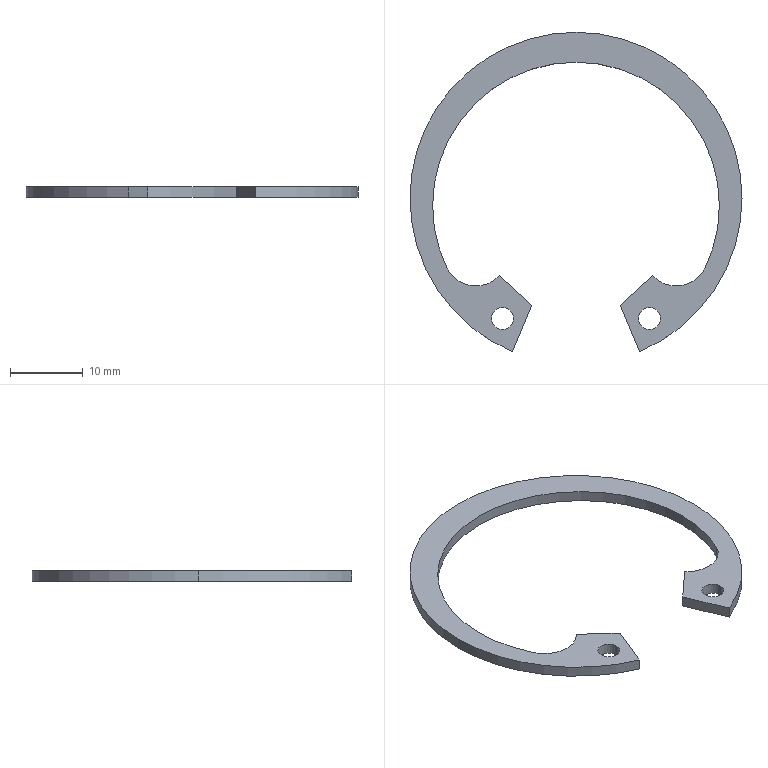Part | STEP file | 1 solid | 18 faces | box 45.5 x 43.768 x 1.5 mm | volume 674.493 mm3 | cylinder 12 | plane 6 | commonest cylinder face diameters 3 x4 39.3 x3 45.5 x3 8.8 x2
STEP:
#1=CARTESIAN_POINT('',(0.,0.,0.));
#2=DIRECTION('',(0.,0.,1.));
#3=DIRECTION('',(1.,0.,0.));
#4=AXIS2_PLACEMENT_3D('',#1,#2,#3);
#5=CARTESIAN_POINT('',(8.568,-16.466,-0.75));
#6=VERTEX_POINT('',#5);
#7=CARTESIAN_POINT('',(11.568,-16.466,-0.75));
#8=VERTEX_POINT('',#7);
#9=CARTESIAN_POINT('',(10.068,-16.466,-0.75));
#10=DIRECTION('',(0.,0.,1.));
#11=DIRECTION('',(-1.,0.,0.));
#12=AXIS2_PLACEMENT_3D('',#9,#10,#11);
#13=CIRCLE('',#12,1.5);
#14=CARTESIAN_POINT('',(0.,0.,-0.75));
#15=DIRECTION('',(0.,0.,1.));
#16=DIRECTION('',(1.,0.,0.));
#17=AXIS2_PLACEMENT_3D('',#14,#15,#16);
#18=PLANE('',#17);
#19=CARTESIAN_POINT('',(10.068,-16.466));
#20=DIRECTION('',(-1.,0.));
#21=AXIS2_PLACEMENT_2D('',#19,#20);
#22=CIRCLE('',#21,1.5);
#23=(GEOMETRIC_REPRESENTATION_CONTEXT(2)PARAMETRIC_REPRESENTATION_CONTEXT()REPRESENTATION_CONTEXT('',''));
#24=DEFINITIONAL_REPRESENTATION('',(#22),#23);
#25=PCURVE('',#18,#24);
#26=CARTESIAN_POINT('',(10.068,-16.466,0.75));
#27=DIRECTION('',(0.,0.,-1.));
#28=DIRECTION('',(-1.,0.,0.));
#29=AXIS2_PLACEMENT_3D('',#26,#27,#28);
#30=CYLINDRICAL_SURFACE('',#29,1.5);
#31=CARTESIAN_POINT('',(6.283,1.5));
#32=DIRECTION('',(-1.,0.));
#33=VECTOR('',#32,1.);
#34=LINE('',#31,#33);
#35=(GEOMETRIC_REPRESENTATION_CONTEXT(2)PARAMETRIC_REPRESENTATION_CONTEXT()REPRESENTATION_CONTEXT('',''));
#36=DEFINITIONAL_REPRESENTATION('',(#34),#35);
#37=PCURVE('',#30,#36);
#38=SURFACE_CURVE('',#13,(#25,#37),.PCURVE_S1.);
#39=EDGE_CURVE('',#6,#8,#38,.T.);
#40=ORIENTED_EDGE('',*,*,#39,.T.);
#41=CARTESIAN_POINT('',(10.068,-16.466,-0.75));
#42=DIRECTION('',(0.,0.,1.));
#43=DIRECTION('',(-1.,0.,0.));
#44=AXIS2_PLACEMENT_3D('',#41,#42,#43);
#45=CIRCLE('',#44,1.5);
#46=CARTESIAN_POINT('',(10.068,-16.466));
#47=DIRECTION('',(-1.,0.));
#48=AXIS2_PLACEMENT_2D('',#46,#47);
#49=CIRCLE('',#48,1.5);
#50=(GEOMETRIC_REPRESENTATION_CONTEXT(2)PARAMETRIC_REPRESENTATION_CONTEXT()REPRESENTATION_CONTEXT('',''));
#51=DEFINITIONAL_REPRESENTATION('',(#49),#50);
#52=PCURVE('',#18,#51);
#53=CARTESIAN_POINT('',(10.068,-16.466,0.75));
#54=DIRECTION('',(0.,0.,-1.));
#55=DIRECTION('',(-1.,0.,0.));
#56=AXIS2_PLACEMENT_3D('',#53,#54,#55);
#57=CYLINDRICAL_SURFACE('',#56,1.5);
#58=CARTESIAN_POINT('',(6.283,1.5));
#59=DIRECTION('',(-1.,0.));
#60=VECTOR('',#59,1.);
#61=LINE('',#58,#60);
#62=(GEOMETRIC_REPRESENTATION_CONTEXT(2)PARAMETRIC_REPRESENTATION_CONTEXT()REPRESENTATION_CONTEXT('',''));
#63=DEFINITIONAL_REPRESENTATION('',(#61),#62);
#64=PCURVE('',#57,#63);
#65=SURFACE_CURVE('',#45,(#52,#64),.PCURVE_S1.);
#66=EDGE_CURVE('',#8,#6,#65,.T.);
#67=ORIENTED_EDGE('',*,*,#66,.T.);
#68=EDGE_LOOP('',(#40,#67));
#69=FACE_BOUND('',#68,.T.);
#70=CARTESIAN_POINT('',(-11.568,-16.466,-0.75));
#71=VERTEX_POINT('',#70);
#72=CARTESIAN_POINT('',(-8.568,-16.466,-0.75));
#73=VERTEX_POINT('',#72);
#74=CARTESIAN_POINT('',(-10.068,-16.466,-0.75));
#75=DIRECTION('',(0.,0.,1.));
#76=DIRECTION('',(-1.,0.,0.));
#77=AXIS2_PLACEMENT_3D('',#74,#75,#76);
#78=CIRCLE('',#77,1.5);
#79=CARTESIAN_POINT('',(-10.068,-16.466));
#80=DIRECTION('',(-1.,0.));
#81=AXIS2_PLACEMENT_2D('',#79,#80);
#82=CIRCLE('',#81,1.5);
#83=(GEOMETRIC_REPRESENTATION_CONTEXT(2)PARAMETRIC_REPRESENTATION_CONTEXT()REPRESENTATION_CONTEXT('',''));
#84=DEFINITIONAL_REPRESENTATION('',(#82),#83);
#85=PCURVE('',#18,#84);
#86=CARTESIAN_POINT('',(-10.068,-16.466,0.75));
#87=DIRECTION('',(0.,0.,-1.));
#88=DIRECTION('',(-1.,0.,0.));
#89=AXIS2_PLACEMENT_3D('',#86,#87,#88);
#90=CYLINDRICAL_SURFACE('',#89,1.5);
#91=CARTESIAN_POINT('',(6.283,1.5));
#92=DIRECTION('',(-1.,0.));
#93=VECTOR('',#92,1.);
#94=LINE('',#91,#93);
#95=(GEOMETRIC_REPRESENTATION_CONTEXT(2)PARAMETRIC_REPRESENTATION_CONTEXT()REPRESENTATION_CONTEXT('',''));
#96=DEFINITIONAL_REPRESENTATION('',(#94),#95);
#97=PCURVE('',#90,#96);
#98=SURFACE_CURVE('',#78,(#85,#97),.PCURVE_S1.);
#99=EDGE_CURVE('',#71,#73,#98,.T.);
#100=ORIENTED_EDGE('',*,*,#99,.T.);
#101=CARTESIAN_POINT('',(-10.068,-16.466,-0.75));
#102=DIRECTION('',(0.,0.,1.));
#103=DIRECTION('',(-1.,0.,0.));
#104=AXIS2_PLACEMENT_3D('',#101,#102,#103);
#105=CIRCLE('',#104,1.5);
#106=CARTESIAN_POINT('',(-10.068,-16.466));
#107=DIRECTION('',(-1.,0.));
#108=AXIS2_PLACEMENT_2D('',#106,#107);
#109=CIRCLE('',#108,1.5);
#110=(GEOMETRIC_REPRESENTATION_CONTEXT(2)PARAMETRIC_REPRESENTATION_CONTEXT()REPRESENTATION_CONTEXT('',''));
#111=DEFINITIONAL_REPRESENTATION('',(#109),#110);
#112=PCURVE('',#18,#111);
#113=CARTESIAN_POINT('',(-10.068,-16.466,0.75));
#114=DIRECTION('',(0.,0.,-1.));
#115=DIRECTION('',(-1.,0.,0.));
#116=AXIS2_PLACEMENT_3D('',#113,#114,#115);
#117=CYLINDRICAL_SURFACE('',#116,1.5);
#118=CARTESIAN_POINT('',(6.283,1.5));
#119=DIRECTION('',(-1.,0.));
#120=VECTOR('',#119,1.);
#121=LINE('',#118,#120);
#122=(GEOMETRIC_REPRESENTATION_CONTEXT(2)PARAMETRIC_REPRESENTATION_CONTEXT()REPRESENTATION_CONTEXT('',''));
#123=DEFINITIONAL_REPRESENTATION('',(#121),#122);
#124=PCURVE('',#117,#123);
#125=SURFACE_CURVE('',#105,(#112,#124),.PCURVE_S1.);
#126=EDGE_CURVE('',#73,#71,#125,.T.);
#127=ORIENTED_EDGE('',*,*,#126,.T.);
#128=EDGE_LOOP('',(#100,#127));
#129=FACE_BOUND('',#128,.T.);
#130=CARTESIAN_POINT('',(8.706,-21.018,-0.75));
#131=VERTEX_POINT('',#130);
#132=CARTESIAN_POINT('',(6.066,-14.643,-0.75));
#133=VERTEX_POINT('',#132);
#134=CARTESIAN_POINT('',(6.066,-14.643,-0.75));
#135=DIRECTION('',(-0.3827,0.9239,0.));
#136=VECTOR('',#135,1.);
#137=LINE('',#134,#136);
#138=CARTESIAN_POINT('',(6.066,-14.643));
#139=DIRECTION('',(-0.3827,0.9239));
#140=VECTOR('',#139,1.);
#141=LINE('',#138,#140);
#142=(GEOMETRIC_REPRESENTATION_CONTEXT(2)PARAMETRIC_REPRESENTATION_CONTEXT()REPRESENTATION_CONTEXT('',''));
#143=DEFINITIONAL_REPRESENTATION('',(#141),#142);
#144=PCURVE('',#18,#143);
#145=CARTESIAN_POINT('',(6.066,-14.643,0.75));
#146=DIRECTION('',(0.9239,0.3827,0.));
#147=DIRECTION('',(0.,0.,-1.));
#148=AXIS2_PLACEMENT_3D('',#145,#146,#147);
#149=PLANE('',#148);
#150=CARTESIAN_POINT('',(1.5,0.));
#151=DIRECTION('',(0.,1.));
#152=VECTOR('',#151,1.);
#153=LINE('',#150,#152);
#154=(GEOMETRIC_REPRESENTATION_CONTEXT(2)PARAMETRIC_REPRESENTATION_CONTEXT()REPRESENTATION_CONTEXT('',''));
#155=DEFINITIONAL_REPRESENTATION('',(#153),#154);
#156=PCURVE('',#149,#155);
#157=SURFACE_CURVE('',#137,(#144,#156),.PCURVE_S1.);
#158=EDGE_CURVE('',#131,#133,#157,.T.);
#159=ORIENTED_EDGE('',*,*,#158,.T.);
#160=CARTESIAN_POINT('',(10.492,-10.593,-0.75));
#161=VERTEX_POINT('',#160);
#162=CARTESIAN_POINT('',(10.492,-10.593,-0.75));
#163=DIRECTION('',(0.7377,0.6752,0.));
#164=VECTOR('',#163,1.);
#165=LINE('',#162,#164);
#166=CARTESIAN_POINT('',(10.492,-10.593));
#167=DIRECTION('',(0.7377,0.6752));
#168=VECTOR('',#167,1.);
#169=LINE('',#166,#168);
#170=(GEOMETRIC_REPRESENTATION_CONTEXT(2)PARAMETRIC_REPRESENTATION_CONTEXT()REPRESENTATION_CONTEXT('',''));
#171=DEFINITIONAL_REPRESENTATION('',(#169),#170);
#172=PCURVE('',#18,#171);
#173=CARTESIAN_POINT('',(10.492,-10.593,0.75));
#174=DIRECTION('',(0.6752,-0.7377,0.));
#175=DIRECTION('',(0.,0.,-1.));
#176=AXIS2_PLACEMENT_3D('',#173,#174,#175);
#177=PLANE('',#176);
#178=CARTESIAN_POINT('',(1.5,0.));
#179=DIRECTION('',(0.,1.));
#180=VECTOR('',#179,1.);
#181=LINE('',#178,#180);
#182=(GEOMETRIC_REPRESENTATION_CONTEXT(2)PARAMETRIC_REPRESENTATION_CONTEXT()REPRESENTATION_CONTEXT('',''));
#183=DEFINITIONAL_REPRESENTATION('',(#181),#182);
#184=PCURVE('',#177,#183);
#185=SURFACE_CURVE('',#165,(#172,#184),.PCURVE_S1.);
#186=EDGE_CURVE('',#133,#161,#185,.T.);
#187=ORIENTED_EDGE('',*,*,#186,.T.);
#188=CARTESIAN_POINT('',(17.701,-9.532,-0.75));
#189=VERTEX_POINT('',#188);
#190=CARTESIAN_POINT('',(13.737,-7.622,-0.75));
#191=DIRECTION('',(0.,0.,1.));
#192=DIRECTION('',(-1.,0.,0.));
#193=AXIS2_PLACEMENT_3D('',#190,#191,#192);
#194=CIRCLE('',#193,4.4);
#195=CARTESIAN_POINT('',(13.737,-7.622));
#196=DIRECTION('',(-1.,0.));
#197=AXIS2_PLACEMENT_2D('',#195,#196);
#198=CIRCLE('',#197,4.4);
#199=(GEOMETRIC_REPRESENTATION_CONTEXT(2)PARAMETRIC_REPRESENTATION_CONTEXT()REPRESENTATION_CONTEXT('',''));
#200=DEFINITIONAL_REPRESENTATION('',(#198),#199);
#201=PCURVE('',#18,#200);
#202=CARTESIAN_POINT('',(13.737,-7.622,0.75));
#203=DIRECTION('',(0.,0.,-1.));
#204=DIRECTION('',(-1.,0.,0.));
#205=AXIS2_PLACEMENT_3D('',#202,#203,#204);
#206=CYLINDRICAL_SURFACE('',#205,4.4);
#207=CARTESIAN_POINT('',(6.283,1.5));
#208=DIRECTION('',(-1.,0.));
#209=VECTOR('',#208,1.);
#210=LINE('',#207,#209);
#211=(GEOMETRIC_REPRESENTATION_CONTEXT(2)PARAMETRIC_REPRESENTATION_CONTEXT()REPRESENTATION_CONTEXT('',''));
#212=DEFINITIONAL_REPRESENTATION('',(#210),#211);
#213=PCURVE('',#206,#212);
#214=SURFACE_CURVE('',#194,(#201,#213),.PCURVE_S1.);
#215=EDGE_CURVE('',#161,#189,#214,.T.);
#216=ORIENTED_EDGE('',*,*,#215,.T.);
#217=CARTESIAN_POINT('',(19.65,-1.,-0.75));
#218=VERTEX_POINT('',#217);
#219=CARTESIAN_POINT('',(0.,-1.,-0.75));
#220=DIRECTION('',(0.,0.,1.));
#221=DIRECTION('',(-1.,0.,0.));
#222=AXIS2_PLACEMENT_3D('',#219,#220,#221);
#223=CIRCLE('',#222,19.65);
#224=CARTESIAN_POINT('',(0.,-1.));
#225=DIRECTION('',(-1.,0.));
#226=AXIS2_PLACEMENT_2D('',#224,#225);
#227=CIRCLE('',#226,19.65);
#228=(GEOMETRIC_REPRESENTATION_CONTEXT(2)PARAMETRIC_REPRESENTATION_CONTEXT()REPRESENTATION_CONTEXT('',''));
#229=DEFINITIONAL_REPRESENTATION('',(#227),#228);
#230=PCURVE('',#18,#229);
#231=CARTESIAN_POINT('',(0.,-1.,0.75));
#232=DIRECTION('',(0.,0.,-1.));
#233=DIRECTION('',(-1.,0.,0.));
#234=AXIS2_PLACEMENT_3D('',#231,#232,#233);
#235=CYLINDRICAL_SURFACE('',#234,19.65);
#236=CARTESIAN_POINT('',(6.283,1.5));
#237=DIRECTION('',(-1.,0.));
#238=VECTOR('',#237,1.);
#239=LINE('',#236,#238);
#240=(GEOMETRIC_REPRESENTATION_CONTEXT(2)PARAMETRIC_REPRESENTATION_CONTEXT()REPRESENTATION_CONTEXT('',''));
#241=DEFINITIONAL_REPRESENTATION('',(#239),#240);
#242=PCURVE('',#235,#241);
#243=SURFACE_CURVE('',#223,(#230,#242),.PCURVE_S1.);
#244=EDGE_CURVE('',#189,#218,#243,.T.);
#245=ORIENTED_EDGE('',*,*,#244,.T.);
#246=CARTESIAN_POINT('',(-19.65,-1.,-0.75));
#247=VERTEX_POINT('',#246);
#248=CARTESIAN_POINT('',(0.,-1.,-0.75));
#249=DIRECTION('',(0.,0.,1.));
#250=DIRECTION('',(-1.,0.,0.));
#251=AXIS2_PLACEMENT_3D('',#248,#249,#250);
#252=CIRCLE('',#251,19.65);
#253=CARTESIAN_POINT('',(0.,-1.));
#254=DIRECTION('',(-1.,0.));
#255=AXIS2_PLACEMENT_2D('',#253,#254);
#256=CIRCLE('',#255,19.65);
#257=(GEOMETRIC_REPRESENTATION_CONTEXT(2)PARAMETRIC_REPRESENTATION_CONTEXT()REPRESENTATION_CONTEXT('',''));
#258=DEFINITIONAL_REPRESENTATION('',(#256),#257);
#259=PCURVE('',#18,#258);
#260=CARTESIAN_POINT('',(0.,-1.,0.75));
#261=DIRECTION('',(0.,0.,-1.));
#262=DIRECTION('',(-1.,0.,0.));
#263=AXIS2_PLACEMENT_3D('',#260,#261,#262);
#264=CYLINDRICAL_SURFACE('',#263,19.65);
#265=CARTESIAN_POINT('',(6.283,1.5));
#266=DIRECTION('',(-1.,0.));
#267=VECTOR('',#266,1.);
#268=LINE('',#265,#267);
#269=(GEOMETRIC_REPRESENTATION_CONTEXT(2)PARAMETRIC_REPRESENTATION_CONTEXT()REPRESENTATION_CONTEXT('',''));
#270=DEFINITIONAL_REPRESENTATION('',(#268),#269);
#271=PCURVE('',#264,#270);
#272=SURFACE_CURVE('',#252,(#259,#271),.PCURVE_S1.);
#273=EDGE_CURVE('',#218,#247,#272,.T.);
#274=ORIENTED_EDGE('',*,*,#273,.T.);
#275=CARTESIAN_POINT('',(-17.701,-9.532,-0.75));
#276=VERTEX_POINT('',#275);
#277=CARTESIAN_POINT('',(0.,-1.,-0.75));
#278=DIRECTION('',(0.,0.,1.));
#279=DIRECTION('',(-1.,0.,0.));
#280=AXIS2_PLACEMENT_3D('',#277,#278,#279);
#281=CIRCLE('',#280,19.65);
#282=CARTESIAN_POINT('',(0.,-1.));
#283=DIRECTION('',(-1.,0.));
#284=AXIS2_PLACEMENT_2D('',#282,#283);
#285=CIRCLE('',#284,19.65);
#286=(GEOMETRIC_REPRESENTATION_CONTEXT(2)PARAMETRIC_REPRESENTATION_CONTEXT()REPRESENTATION_CONTEXT('',''));
#287=DEFINITIONAL_REPRESENTATION('',(#285),#286);
#288=PCURVE('',#18,#287);
#289=CARTESIAN_POINT('',(0.,-1.,0.75));
#290=DIRECTION('',(0.,0.,-1.));
#291=DIRECTION('',(-1.,0.,0.));
#292=AXIS2_PLACEMENT_3D('',#289,#290,#291);
#293=CYLINDRICAL_SURFACE('',#292,19.65);
#294=CARTESIAN_POINT('',(6.283,1.5));
#295=DIRECTION('',(-1.,0.));
#296=VECTOR('',#295,1.);
#297=LINE('',#294,#296);
#298=(GEOMETRIC_REPRESENTATION_CONTEXT(2)PARAMETRIC_REPRESENTATION_CONTEXT()REPRESENTATION_CONTEXT('',''));
#299=DEFINITIONAL_REPRESENTATION('',(#297),#298);
#300=PCURVE('',#293,#299);
#301=SURFACE_CURVE('',#281,(#288,#300),.PCURVE_S1.);
#302=EDGE_CURVE('',#247,#276,#301,.T.);
#303=ORIENTED_EDGE('',*,*,#302,.T.);
#304=CARTESIAN_POINT('',(-10.492,-10.593,-0.75));
#305=VERTEX_POINT('',#304);
#306=CARTESIAN_POINT('',(-13.737,-7.622,-0.75));
#307=DIRECTION('',(0.,0.,1.));
#308=DIRECTION('',(-1.,0.,0.));
#309=AXIS2_PLACEMENT_3D('',#306,#307,#308);
#310=CIRCLE('',#309,4.4);
#311=CARTESIAN_POINT('',(-13.737,-7.622));
#312=DIRECTION('',(-1.,0.));
#313=AXIS2_PLACEMENT_2D('',#311,#312);
#314=CIRCLE('',#313,4.4);
#315=(GEOMETRIC_REPRESENTATION_CONTEXT(2)PARAMETRIC_REPRESENTATION_CONTEXT()REPRESENTATION_CONTEXT('',''));
#316=DEFINITIONAL_REPRESENTATION('',(#314),#315);
#317=PCURVE('',#18,#316);
#318=CARTESIAN_POINT('',(-13.737,-7.622,0.75));
#319=DIRECTION('',(0.,0.,-1.));
#320=DIRECTION('',(-1.,0.,0.));
#321=AXIS2_PLACEMENT_3D('',#318,#319,#320);
#322=CYLINDRICAL_SURFACE('',#321,4.4);
#323=CARTESIAN_POINT('',(6.283,1.5));
#324=DIRECTION('',(-1.,0.));
#325=VECTOR('',#324,1.);
#326=LINE('',#323,#325);
#327=(GEOMETRIC_REPRESENTATION_CONTEXT(2)PARAMETRIC_REPRESENTATION_CONTEXT()REPRESENTATION_CONTEXT('',''));
#328=DEFINITIONAL_REPRESENTATION('',(#326),#327);
#329=PCURVE('',#322,#328);
#330=SURFACE_CURVE('',#310,(#317,#329),.PCURVE_S1.);
#331=EDGE_CURVE('',#276,#305,#330,.T.);
#332=ORIENTED_EDGE('',*,*,#331,.T.);
#333=CARTESIAN_POINT('',(-6.066,-14.643,-0.75));
#334=VERTEX_POINT('',#333);
#335=CARTESIAN_POINT('',(-10.492,-10.593,-0.75));
#336=DIRECTION('',(0.7377,-0.6752,0.));
#337=VECTOR('',#336,1.);
#338=LINE('',#335,#337);
#339=CARTESIAN_POINT('',(-10.492,-10.593));
#340=DIRECTION('',(0.7377,-0.6752));
#341=VECTOR('',#340,1.);
#342=LINE('',#339,#341);
#343=(GEOMETRIC_REPRESENTATION_CONTEXT(2)PARAMETRIC_REPRESENTATION_CONTEXT()REPRESENTATION_CONTEXT('',''));
#344=DEFINITIONAL_REPRESENTATION('',(#342),#343);
#345=PCURVE('',#18,#344);
#346=CARTESIAN_POINT('',(-10.492,-10.593,0.75));
#347=DIRECTION('',(-0.6752,-0.7377,0.));
#348=DIRECTION('',(-0.7377,0.6752,0.));
#349=AXIS2_PLACEMENT_3D('',#346,#347,#348);
#350=PLANE('',#349);
#351=CARTESIAN_POINT('',(0.,1.5));
#352=DIRECTION('',(-1.,0.));
#353=VECTOR('',#352,1.);
#354=LINE('',#351,#353);
#355=(GEOMETRIC_REPRESENTATION_CONTEXT(2)PARAMETRIC_REPRESENTATION_CONTEXT()REPRESENTATION_CONTEXT('',''));
#356=DEFINITIONAL_REPRESENTATION('',(#354),#355);
#357=PCURVE('',#350,#356);
#358=SURFACE_CURVE('',#338,(#345,#357),.PCURVE_S1.);
#359=EDGE_CURVE('',#305,#334,#358,.T.);
#360=ORIENTED_EDGE('',*,*,#359,.T.);
#361=CARTESIAN_POINT('',(-8.706,-21.018,-0.75));
#362=VERTEX_POINT('',#361);
#363=CARTESIAN_POINT('',(-6.066,-14.643,-0.75));
#364=DIRECTION('',(-0.3827,-0.9239,0.));
#365=VECTOR('',#364,1.);
#366=LINE('',#363,#365);
#367=CARTESIAN_POINT('',(-6.066,-14.643));
#368=DIRECTION('',(-0.3827,-0.9239));
#369=VECTOR('',#368,1.);
#370=LINE('',#367,#369);
#371=(GEOMETRIC_REPRESENTATION_CONTEXT(2)PARAMETRIC_REPRESENTATION_CONTEXT()REPRESENTATION_CONTEXT('',''));
#372=DEFINITIONAL_REPRESENTATION('',(#370),#371);
#373=PCURVE('',#18,#372);
#374=CARTESIAN_POINT('',(-6.066,-14.643,0.75));
#375=DIRECTION('',(-0.9239,0.3827,0.));
#376=DIRECTION('',(0.,0.,1.));
#377=AXIS2_PLACEMENT_3D('',#374,#375,#376);
#378=PLANE('',#377);
#379=CARTESIAN_POINT('',(-1.5,0.));
#380=DIRECTION('',(0.,-1.));
#381=VECTOR('',#380,1.);
#382=LINE('',#379,#381);
#383=(GEOMETRIC_REPRESENTATION_CONTEXT(2)PARAMETRIC_REPRESENTATION_CONTEXT()REPRESENTATION_CONTEXT('',''));
#384=DEFINITIONAL_REPRESENTATION('',(#382),#383);
#385=PCURVE('',#378,#384);
#386=SURFACE_CURVE('',#366,(#373,#385),.PCURVE_S1.);
#387=EDGE_CURVE('',#334,#362,#386,.T.);
#388=ORIENTED_EDGE('',*,*,#387,.T.);
#389=CARTESIAN_POINT('',(-22.75,0.,-0.75));
#390=VERTEX_POINT('',#389);
#391=CARTESIAN_POINT('',(0.,0.,-0.75));
#392=DIRECTION('',(0.,0.,1.));
#393=DIRECTION('',(-1.,0.,0.));
#394=AXIS2_PLACEMENT_3D('',#391,#392,#393);
#395=CIRCLE('',#394,22.75);
#396=CARTESIAN_POINT('',(0.,0.));
#397=DIRECTION('',(-1.,0.));
#398=AXIS2_PLACEMENT_2D('',#396,#397);
#399=CIRCLE('',#398,22.75);
#400=(GEOMETRIC_REPRESENTATION_CONTEXT(2)PARAMETRIC_REPRESENTATION_CONTEXT()REPRESENTATION_CONTEXT('',''));
#401=DEFINITIONAL_REPRESENTATION('',(#399),#400);
#402=PCURVE('',#18,#401);
#403=CARTESIAN_POINT('',(0.,0.,0.75));
#404=DIRECTION('',(0.,0.,-1.));
#405=DIRECTION('',(-1.,0.,0.));
#406=AXIS2_PLACEMENT_3D('',#403,#404,#405);
#407=CYLINDRICAL_SURFACE('',#406,22.75);
#408=CARTESIAN_POINT('',(6.283,1.5));
#409=DIRECTION('',(-1.,0.));
#410=VECTOR('',#409,1.);
#411=LINE('',#408,#410);
#412=(GEOMETRIC_REPRESENTATION_CONTEXT(2)PARAMETRIC_REPRESENTATION_CONTEXT()REPRESENTATION_CONTEXT('',''));
#413=DEFINITIONAL_REPRESENTATION('',(#411),#412);
#414=PCURVE('',#407,#413);
#415=SURFACE_CURVE('',#395,(#402,#414),.PCURVE_S1.);
#416=EDGE_CURVE('',#390,#362,#415,.T.);
#417=ORIENTED_EDGE('',*,*,#416,.F.);
#418=CARTESIAN_POINT('',(22.75,0.,-0.75));
#419=VERTEX_POINT('',#418);
#420=CARTESIAN_POINT('',(0.,0.,-0.75));
#421=DIRECTION('',(0.,0.,1.));
#422=DIRECTION('',(-1.,0.,0.));
#423=AXIS2_PLACEMENT_3D('',#420,#421,#422);
#424=CIRCLE('',#423,22.75);
#425=CARTESIAN_POINT('',(0.,0.));
#426=DIRECTION('',(-1.,0.));
#427=AXIS2_PLACEMENT_2D('',#425,#426);
#428=CIRCLE('',#427,22.75);
#429=(GEOMETRIC_REPRESENTATION_CONTEXT(2)PARAMETRIC_REPRESENTATION_CONTEXT()REPRESENTATION_CONTEXT('',''));
#430=DEFINITIONAL_REPRESENTATION('',(#428),#429);
#431=PCURVE('',#18,#430);
#432=CARTESIAN_POINT('',(0.,0.,0.75));
#433=DIRECTION('',(0.,0.,-1.));
#434=DIRECTION('',(-1.,0.,0.));
#435=AXIS2_PLACEMENT_3D('',#432,#433,#434);
#436=CYLINDRICAL_SURFACE('',#435,22.75);
#437=CARTESIAN_POINT('',(6.283,1.5));
#438=DIRECTION('',(-1.,0.));
#439=VECTOR('',#438,1.);
#440=LINE('',#437,#439);
#441=(GEOMETRIC_REPRESENTATION_CONTEXT(2)PARAMETRIC_REPRESENTATION_CONTEXT()REPRESENTATION_CONTEXT('',''));
#442=DEFINITIONAL_REPRESENTATION('',(#440),#441);
#443=PCURVE('',#436,#442);
#444=SURFACE_CURVE('',#424,(#431,#443),.PCURVE_S1.);
#445=EDGE_CURVE('',#419,#390,#444,.T.);
#446=ORIENTED_EDGE('',*,*,#445,.F.);
#447=CARTESIAN_POINT('',(0.,0.,-0.75));
#448=DIRECTION('',(0.,0.,1.));
#449=DIRECTION('',(-1.,0.,0.));
#450=AXIS2_PLACEMENT_3D('',#447,#448,#449);
#451=CIRCLE('',#450,22.75);
#452=CARTESIAN_POINT('',(0.,0.));
#453=DIRECTION('',(-1.,0.));
#454=AXIS2_PLACEMENT_2D('',#452,#453);
#455=CIRCLE('',#454,22.75);
#456=(GEOMETRIC_REPRESENTATION_CONTEXT(2)PARAMETRIC_REPRESENTATION_CONTEXT()REPRESENTATION_CONTEXT('',''));
#457=DEFINITIONAL_REPRESENTATION('',(#455),#456);
#458=PCURVE('',#18,#457);
#459=CARTESIAN_POINT('',(0.,0.,0.75));
#460=DIRECTION('',(0.,0.,-1.));
#461=DIRECTION('',(-1.,0.,0.));
#462=AXIS2_PLACEMENT_3D('',#459,#460,#461);
#463=CYLINDRICAL_SURFACE('',#462,22.75);
#464=CARTESIAN_POINT('',(6.283,1.5));
#465=DIRECTION('',(-1.,0.));
#466=VECTOR('',#465,1.);
#467=LINE('',#464,#466);
#468=(GEOMETRIC_REPRESENTATION_CONTEXT(2)PARAMETRIC_REPRESENTATION_CONTEXT()REPRESENTATION_CONTEXT('',''));
#469=DEFINITIONAL_REPRESENTATION('',(#467),#468);
#470=PCURVE('',#463,#469);
#471=SURFACE_CURVE('',#451,(#458,#470),.PCURVE_S1.);
#472=EDGE_CURVE('',#131,#419,#471,.T.);
#473=ORIENTED_EDGE('',*,*,#472,.F.);
#474=EDGE_LOOP('',(#159,#187,#216,#245,#274,#303,#332,#360,#388,#417,#446,#473));
#475=FACE_BOUND('',#474,.T.);
#476=ADVANCED_FACE('',(#69,#129,#475),#18,.F.);
#477=ORIENTED_EDGE('',*,*,#126,.T.);
#478=CARTESIAN_POINT('',(-11.568,-16.466,0.75));
#479=VERTEX_POINT('',#478);
#480=CARTESIAN_POINT('',(-11.568,-16.466,0.75));
#481=DIRECTION('',(0.,0.,-1.));
#482=VECTOR('',#481,1.);
#483=LINE('',#480,#482);
#484=CARTESIAN_POINT('',(0.,0.));
#485=DIRECTION('',(0.,1.));
#486=VECTOR('',#485,1.);
#487=LINE('',#484,#486);
#488=(GEOMETRIC_REPRESENTATION_CONTEXT(2)PARAMETRIC_REPRESENTATION_CONTEXT()REPRESENTATION_CONTEXT('',''));
#489=DEFINITIONAL_REPRESENTATION('',(#487),#488);
#490=PCURVE('',#117,#489);
#491=CARTESIAN_POINT('',(6.283,0.));
#492=DIRECTION('',(0.,1.));
#493=VECTOR('',#492,1.);
#494=LINE('',#491,#493);
#495=(GEOMETRIC_REPRESENTATION_CONTEXT(2)PARAMETRIC_REPRESENTATION_CONTEXT()REPRESENTATION_CONTEXT('',''));
#496=DEFINITIONAL_REPRESENTATION('',(#494),#495);
#497=PCURVE('',#90,#496);
#498=SURFACE_CURVE('',#483,(#490,#497),.PCURVE_S1.);
#499=EDGE_CURVE('',#479,#71,#498,.T.);
#500=ORIENTED_EDGE('',*,*,#499,.F.);
#501=CARTESIAN_POINT('',(-8.568,-16.466,0.75));
#502=VERTEX_POINT('',#501);
#503=CARTESIAN_POINT('',(-10.068,-16.466,0.75));
#504=DIRECTION('',(0.,0.,-1.));
#505=DIRECTION('',(-1.,0.,0.));
#506=AXIS2_PLACEMENT_3D('',#503,#504,#505);
#507=CIRCLE('',#506,1.5);
#508=CARTESIAN_POINT('',(0.,0.));
#509=DIRECTION('',(1.,0.));
#510=VECTOR('',#509,1.);
#511=LINE('',#508,#510);
#512=(GEOMETRIC_REPRESENTATION_CONTEXT(2)PARAMETRIC_REPRESENTATION_CONTEXT()REPRESENTATION_CONTEXT('',''));
#513=DEFINITIONAL_REPRESENTATION('',(#511),#512);
#514=PCURVE('',#117,#513);
#515=CARTESIAN_POINT('',(0.,0.,0.75));
#516=DIRECTION('',(0.,0.,1.));
#517=DIRECTION('',(1.,0.,0.));
#518=AXIS2_PLACEMENT_3D('',#515,#516,#517);
#519=PLANE('',#518);
#520=CARTESIAN_POINT('',(-11.568,-16.466));
#521=CARTESIAN_POINT('',(-11.568,-13.868));
#522=CARTESIAN_POINT('',(-9.318,-15.167));
#523=CARTESIAN_POINT('',(-7.068,-16.466));
#524=CARTESIAN_POINT('',(-9.318,-17.765));
#525=CARTESIAN_POINT('',(-11.568,-19.064));
#526=CARTESIAN_POINT('',(-11.568,-16.466));
#527=(BOUNDED_CURVE()B_SPLINE_CURVE(2,(#520,#521,#522,#523,#524,#525,#526),.UNSPECIFIED.,.T.,.F.)B_SPLINE_CURVE_WITH_KNOTS((1,2,2,2,2,1),(-2.094,0.,2.094,4.189,6.283,8.378),.UNSPECIFIED.)CURVE()GEOMETRIC_REPRESENTATION_ITEM()RATIONAL_B_SPLINE_CURVE((1.,0.5,1.,0.5,1.,0.5,1.))REPRESENTATION_ITEM(''));
#528=(GEOMETRIC_REPRESENTATION_CONTEXT(2)PARAMETRIC_REPRESENTATION_CONTEXT()REPRESENTATION_CONTEXT('',''));
#529=DEFINITIONAL_REPRESENTATION('',(#527),#528);
#530=PCURVE('',#519,#529);
#531=SURFACE_CURVE('',#507,(#514,#530),.PCURVE_S1.);
#532=EDGE_CURVE('',#479,#502,#531,.T.);
#533=ORIENTED_EDGE('',*,*,#532,.T.);
#534=CARTESIAN_POINT('',(-8.568,-16.466,0.75));
#535=DIRECTION('',(0.,0.,-1.));
#536=VECTOR('',#535,1.);
#537=LINE('',#534,#536);
#538=CARTESIAN_POINT('',(3.142,0.));
#539=DIRECTION('',(0.,1.));
#540=VECTOR('',#539,1.);
#541=LINE('',#538,#540);
#542=(GEOMETRIC_REPRESENTATION_CONTEXT(2)PARAMETRIC_REPRESENTATION_CONTEXT()REPRESENTATION_CONTEXT('',''));
#543=DEFINITIONAL_REPRESENTATION('',(#541),#542);
#544=PCURVE('',#117,#543);
#545=CARTESIAN_POINT('',(3.142,0.));
#546=DIRECTION('',(0.,1.));
#547=VECTOR('',#546,1.);
#548=LINE('',#545,#547);
#549=(GEOMETRIC_REPRESENTATION_CONTEXT(2)PARAMETRIC_REPRESENTATION_CONTEXT()REPRESENTATION_CONTEXT('',''));
#550=DEFINITIONAL_REPRESENTATION('',(#548),#549);
#551=PCURVE('',#90,#550);
#552=SURFACE_CURVE('',#537,(#544,#551),.PCURVE_S1.);
#553=EDGE_CURVE('',#502,#73,#552,.T.);
#554=ORIENTED_EDGE('',*,*,#553,.T.);
#555=EDGE_LOOP('',(#477,#500,#533,#554));
#556=FACE_BOUND('',#555,.F.);
#557=ADVANCED_FACE('',(#556),#117,.F.);
#558=CARTESIAN_POINT('',(22.75,0.,0.75));
#559=VERTEX_POINT('',#558);
#560=CARTESIAN_POINT('',(22.75,0.,0.75));
#561=DIRECTION('',(0.,0.,-1.));
#562=VECTOR('',#561,1.);
#563=LINE('',#560,#562);
#564=CARTESIAN_POINT('',(3.142,0.));
#565=DIRECTION('',(0.,1.));
#566=VECTOR('',#565,1.);
#567=LINE('',#564,#566);
#568=(GEOMETRIC_REPRESENTATION_CONTEXT(2)PARAMETRIC_REPRESENTATION_CONTEXT()REPRESENTATION_CONTEXT('',''));
#569=DEFINITIONAL_REPRESENTATION('',(#567),#568);
#570=PCURVE('',#463,#569);
#571=CARTESIAN_POINT('',(3.142,0.));
#572=DIRECTION('',(0.,1.));
#573=VECTOR('',#572,1.);
#574=LINE('',#571,#573);
#575=(GEOMETRIC_REPRESENTATION_CONTEXT(2)PARAMETRIC_REPRESENTATION_CONTEXT()REPRESENTATION_CONTEXT('',''));
#576=DEFINITIONAL_REPRESENTATION('',(#574),#575);
#577=PCURVE('',#436,#576);
#578=SURFACE_CURVE('',#563,(#570,#577),.PCURVE_S1.);
#579=EDGE_CURVE('',#559,#419,#578,.T.);
#580=ORIENTED_EDGE('',*,*,#579,.F.);
#581=CARTESIAN_POINT('',(8.706,-21.018,0.75));
#582=VERTEX_POINT('',#581);
#583=CARTESIAN_POINT('',(0.,0.,0.75));
#584=DIRECTION('',(0.,0.,1.));
#585=DIRECTION('',(-1.,0.,0.));
#586=AXIS2_PLACEMENT_3D('',#583,#584,#585);
#587=CIRCLE('',#586,22.75);
#588=CARTESIAN_POINT('',(6.283,0.));
#589=DIRECTION('',(-1.,0.));
#590=VECTOR('',#589,1.);
#591=LINE('',#588,#590);
#592=(GEOMETRIC_REPRESENTATION_CONTEXT(2)PARAMETRIC_REPRESENTATION_CONTEXT()REPRESENTATION_CONTEXT('',''));
#593=DEFINITIONAL_REPRESENTATION('',(#591),#592);
#594=PCURVE('',#463,#593);
#595=CARTESIAN_POINT('',(0.,0.));
#596=DIRECTION('',(-1.,0.));
#597=AXIS2_PLACEMENT_2D('',#595,#596);
#598=CIRCLE('',#597,22.75);
#599=(GEOMETRIC_REPRESENTATION_CONTEXT(2)PARAMETRIC_REPRESENTATION_CONTEXT()REPRESENTATION_CONTEXT('',''));
#600=DEFINITIONAL_REPRESENTATION('',(#598),#599);
#601=PCURVE('',#519,#600);
#602=SURFACE_CURVE('',#587,(#594,#601),.PCURVE_S1.);
#603=EDGE_CURVE('',#582,#559,#602,.T.);
#604=ORIENTED_EDGE('',*,*,#603,.F.);
#605=CARTESIAN_POINT('',(8.706,-21.018,0.75));
#606=DIRECTION('',(0.,0.,-1.));
#607=VECTOR('',#606,1.);
#608=LINE('',#605,#607);
#609=CARTESIAN_POINT('',(4.32,0.));
#610=DIRECTION('',(0.,1.));
#611=VECTOR('',#610,1.);
#612=LINE('',#609,#611);
#613=(GEOMETRIC_REPRESENTATION_CONTEXT(2)PARAMETRIC_REPRESENTATION_CONTEXT()REPRESENTATION_CONTEXT('',''));
#614=DEFINITIONAL_REPRESENTATION('',(#612),#613);
#615=PCURVE('',#463,#614);
#616=CARTESIAN_POINT('',(0.,-6.9));
#617=DIRECTION('',(1.,0.));
#618=VECTOR('',#617,1.);
#619=LINE('',#616,#618);
#620=(GEOMETRIC_REPRESENTATION_CONTEXT(2)PARAMETRIC_REPRESENTATION_CONTEXT()REPRESENTATION_CONTEXT('',''));
#621=DEFINITIONAL_REPRESENTATION('',(#619),#620);
#622=PCURVE('',#149,#621);
#623=SURFACE_CURVE('',#608,(#615,#622),.PCURVE_S1.);
#624=EDGE_CURVE('',#582,#131,#623,.T.);
#625=ORIENTED_EDGE('',*,*,#624,.T.);
#626=ORIENTED_EDGE('',*,*,#472,.T.);
#627=EDGE_LOOP('',(#580,#604,#625,#626));
#628=FACE_BOUND('',#627,.T.);
#629=ADVANCED_FACE('',(#628),#463,.T.);
#630=ORIENTED_EDGE('',*,*,#387,.F.);
#631=CARTESIAN_POINT('',(-6.066,-14.643,0.75));
#632=VERTEX_POINT('',#631);
#633=CARTESIAN_POINT('',(-6.066,-14.643,0.75));
#634=DIRECTION('',(0.,0.,1.));
#635=VECTOR('',#634,1.);
#636=LINE('',#633,#635);
#637=CARTESIAN_POINT('',(0.,0.));
#638=DIRECTION('',(1.,0.));
#639=VECTOR('',#638,1.);
#640=LINE('',#637,#639);
#641=(GEOMETRIC_REPRESENTATION_CONTEXT(2)PARAMETRIC_REPRESENTATION_CONTEXT()REPRESENTATION_CONTEXT('',''));
#642=DEFINITIONAL_REPRESENTATION('',(#640),#641);
#643=PCURVE('',#378,#642);
#644=CARTESIAN_POINT('',(-6.,0.));
#645=DIRECTION('',(0.,-1.));
#646=VECTOR('',#645,1.);
#647=LINE('',#644,#646);
#648=(GEOMETRIC_REPRESENTATION_CONTEXT(2)PARAMETRIC_REPRESENTATION_CONTEXT()REPRESENTATION_CONTEXT('',''));
#649=DEFINITIONAL_REPRESENTATION('',(#647),#648);
#650=PCURVE('',#350,#649);
#651=SURFACE_CURVE('',#636,(#643,#650),.PCURVE_S1.);
#652=EDGE_CURVE('',#334,#632,#651,.T.);
#653=ORIENTED_EDGE('',*,*,#652,.T.);
#654=CARTESIAN_POINT('',(-8.706,-21.018,0.75));
#655=VERTEX_POINT('',#654);
#656=CARTESIAN_POINT('',(-8.706,-21.018,0.75));
#657=DIRECTION('',(0.3827,0.9239,0.));
#658=VECTOR('',#657,1.);
#659=LINE('',#656,#658);
#660=CARTESIAN_POINT('',(0.,-6.9));
#661=DIRECTION('',(0.,1.));
#662=VECTOR('',#661,1.);
#663=LINE('',#660,#662);
#664=(GEOMETRIC_REPRESENTATION_CONTEXT(2)PARAMETRIC_REPRESENTATION_CONTEXT()REPRESENTATION_CONTEXT('',''));
#665=DEFINITIONAL_REPRESENTATION('',(#663),#664);
#666=PCURVE('',#378,#665);
#667=CARTESIAN_POINT('',(-8.706,-21.018));
#668=DIRECTION('',(0.3827,0.9239));
#669=VECTOR('',#668,1.);
#670=LINE('',#667,#669);
#671=(GEOMETRIC_REPRESENTATION_CONTEXT(2)PARAMETRIC_REPRESENTATION_CONTEXT()REPRESENTATION_CONTEXT('',''));
#672=DEFINITIONAL_REPRESENTATION('',(#670),#671);
#673=PCURVE('',#519,#672);
#674=SURFACE_CURVE('',#659,(#666,#673),.PCURVE_S1.);
#675=EDGE_CURVE('',#655,#632,#674,.T.);
#676=ORIENTED_EDGE('',*,*,#675,.F.);
#677=CARTESIAN_POINT('',(-8.706,-21.018,0.75));
#678=DIRECTION('',(0.,0.,1.));
#679=VECTOR('',#678,1.);
#680=LINE('',#677,#679);
#681=CARTESIAN_POINT('',(0.,-6.9));
#682=DIRECTION('',(1.,0.));
#683=VECTOR('',#682,1.);
#684=LINE('',#681,#683);
#685=(GEOMETRIC_REPRESENTATION_CONTEXT(2)PARAMETRIC_REPRESENTATION_CONTEXT()REPRESENTATION_CONTEXT('',''));
#686=DEFINITIONAL_REPRESENTATION('',(#684),#685);
#687=PCURVE('',#378,#686);
#688=CARTESIAN_POINT('',(5.105,0.));
#689=DIRECTION('',(0.,-1.));
#690=VECTOR('',#689,1.);
#691=LINE('',#688,#690);
#692=(GEOMETRIC_REPRESENTATION_CONTEXT(2)PARAMETRIC_REPRESENTATION_CONTEXT()REPRESENTATION_CONTEXT('',''));
#693=DEFINITIONAL_REPRESENTATION('',(#691),#692);
#694=PCURVE('',#407,#693);
#695=SURFACE_CURVE('',#680,(#687,#694),.PCURVE_S1.);
#696=EDGE_CURVE('',#362,#655,#695,.T.);
#697=ORIENTED_EDGE('',*,*,#696,.F.);
#698=EDGE_LOOP('',(#630,#653,#676,#697));
#699=FACE_BOUND('',#698,.T.);
#700=ADVANCED_FACE('',(#699),#378,.F.);
#701=ORIENTED_EDGE('',*,*,#359,.F.);
#702=CARTESIAN_POINT('',(-10.492,-10.593,0.75));
#703=VERTEX_POINT('',#702);
#704=CARTESIAN_POINT('',(-10.492,-10.593,0.75));
#705=DIRECTION('',(0.,0.,1.));
#706=VECTOR('',#705,1.);
#707=LINE('',#704,#706);
#708=CARTESIAN_POINT('',(0.,0.));
#709=DIRECTION('',(0.,-1.));
#710=VECTOR('',#709,1.);
#711=LINE('',#708,#710);
#712=(GEOMETRIC_REPRESENTATION_CONTEXT(2)PARAMETRIC_REPRESENTATION_CONTEXT()REPRESENTATION_CONTEXT('',''));
#713=DEFINITIONAL_REPRESENTATION('',(#711),#712);
#714=PCURVE('',#350,#713);
#715=CARTESIAN_POINT('',(3.883,0.));
#716=DIRECTION('',(0.,-1.));
#717=VECTOR('',#716,1.);
#718=LINE('',#715,#717);
#719=(GEOMETRIC_REPRESENTATION_CONTEXT(2)PARAMETRIC_REPRESENTATION_CONTEXT()REPRESENTATION_CONTEXT('',''));
#720=DEFINITIONAL_REPRESENTATION('',(#718),#719);
#721=PCURVE('',#322,#720);
#722=SURFACE_CURVE('',#707,(#714,#721),.PCURVE_S1.);
#723=EDGE_CURVE('',#305,#703,#722,.T.);
#724=ORIENTED_EDGE('',*,*,#723,.T.);
#725=CARTESIAN_POINT('',(-6.066,-14.643,0.75));
#726=DIRECTION('',(-0.7377,0.6752,0.));
#727=VECTOR('',#726,1.);
#728=LINE('',#725,#727);
#729=CARTESIAN_POINT('',(-6.,0.));
#730=DIRECTION('',(1.,0.));
#731=VECTOR('',#730,1.);
#732=LINE('',#729,#731);
#733=(GEOMETRIC_REPRESENTATION_CONTEXT(2)PARAMETRIC_REPRESENTATION_CONTEXT()REPRESENTATION_CONTEXT('',''));
#734=DEFINITIONAL_REPRESENTATION('',(#732),#733);
#735=PCURVE('',#350,#734);
#736=CARTESIAN_POINT('',(-6.066,-14.643));
#737=DIRECTION('',(-0.7377,0.6752));
#738=VECTOR('',#737,1.);
#739=LINE('',#736,#738);
#740=(GEOMETRIC_REPRESENTATION_CONTEXT(2)PARAMETRIC_REPRESENTATION_CONTEXT()REPRESENTATION_CONTEXT('',''));
#741=DEFINITIONAL_REPRESENTATION('',(#739),#740);
#742=PCURVE('',#519,#741);
#743=SURFACE_CURVE('',#728,(#735,#742),.PCURVE_S1.);
#744=EDGE_CURVE('',#632,#703,#743,.T.);
#745=ORIENTED_EDGE('',*,*,#744,.F.);
#746=ORIENTED_EDGE('',*,*,#652,.F.);
#747=EDGE_LOOP('',(#701,#724,#745,#746));
#748=FACE_BOUND('',#747,.T.);
#749=ADVANCED_FACE('',(#748),#350,.F.);
#750=ORIENTED_EDGE('',*,*,#723,.T.);
#751=CARTESIAN_POINT('',(-17.701,-9.532,0.75));
#752=VERTEX_POINT('',#751);
#753=CARTESIAN_POINT('',(-13.737,-7.622,0.75));
#754=DIRECTION('',(0.,0.,-1.));
#755=DIRECTION('',(-1.,0.,0.));
#756=AXIS2_PLACEMENT_3D('',#753,#754,#755);
#757=CIRCLE('',#756,4.4);
#758=CARTESIAN_POINT('',(0.,0.));
#759=DIRECTION('',(1.,0.));
#760=VECTOR('',#759,1.);
#761=LINE('',#758,#760);
#762=(GEOMETRIC_REPRESENTATION_CONTEXT(2)PARAMETRIC_REPRESENTATION_CONTEXT()REPRESENTATION_CONTEXT('',''));
#763=DEFINITIONAL_REPRESENTATION('',(#761),#762);
#764=PCURVE('',#322,#763);
#765=CARTESIAN_POINT('',(-18.137,-7.622));
#766=CARTESIAN_POINT('',(-18.137,-0.000806));
#767=CARTESIAN_POINT('',(-11.537,-3.811));
#768=CARTESIAN_POINT('',(-4.937,-7.622));
#769=CARTESIAN_POINT('',(-11.537,-11.432));
#770=CARTESIAN_POINT('',(-18.137,-15.243));
#771=CARTESIAN_POINT('',(-18.137,-7.622));
#772=(BOUNDED_CURVE()B_SPLINE_CURVE(2,(#765,#766,#767,#768,#769,#770,#771),.UNSPECIFIED.,.T.,.F.)B_SPLINE_CURVE_WITH_KNOTS((1,2,2,2,2,1),(-2.094,0.,2.094,4.189,6.283,8.378),.UNSPECIFIED.)CURVE()GEOMETRIC_REPRESENTATION_ITEM()RATIONAL_B_SPLINE_CURVE((1.,0.5,1.,0.5,1.,0.5,1.))REPRESENTATION_ITEM(''));
#773=(GEOMETRIC_REPRESENTATION_CONTEXT(2)PARAMETRIC_REPRESENTATION_CONTEXT()REPRESENTATION_CONTEXT('',''));
#774=DEFINITIONAL_REPRESENTATION('',(#772),#773);
#775=PCURVE('',#519,#774);
#776=SURFACE_CURVE('',#757,(#764,#775),.PCURVE_S1.);
#777=EDGE_CURVE('',#703,#752,#776,.T.);
#778=ORIENTED_EDGE('',*,*,#777,.T.);
#779=CARTESIAN_POINT('',(-17.701,-9.532,0.75));
#780=DIRECTION('',(0.,0.,1.));
#781=VECTOR('',#780,1.);
#782=LINE('',#779,#781);
#783=CARTESIAN_POINT('',(5.834,0.));
#784=DIRECTION('',(0.,-1.));
#785=VECTOR('',#784,1.);
#786=LINE('',#783,#785);
#787=(GEOMETRIC_REPRESENTATION_CONTEXT(2)PARAMETRIC_REPRESENTATION_CONTEXT()REPRESENTATION_CONTEXT('',''));
#788=DEFINITIONAL_REPRESENTATION('',(#786),#787);
#789=PCURVE('',#322,#788);
#790=CARTESIAN_POINT('',(5.834,0.));
#791=DIRECTION('',(0.,-1.));
#792=VECTOR('',#791,1.);
#793=LINE('',#790,#792);
#794=(GEOMETRIC_REPRESENTATION_CONTEXT(2)PARAMETRIC_REPRESENTATION_CONTEXT()REPRESENTATION_CONTEXT('',''));
#795=DEFINITIONAL_REPRESENTATION('',(#793),#794);
#796=PCURVE('',#293,#795);
#797=SURFACE_CURVE('',#782,(#789,#796),.PCURVE_S1.);
#798=EDGE_CURVE('',#276,#752,#797,.T.);
#799=ORIENTED_EDGE('',*,*,#798,.F.);
#800=ORIENTED_EDGE('',*,*,#331,.T.);
#801=EDGE_LOOP('',(#750,#778,#799,#800));
#802=FACE_BOUND('',#801,.F.);
#803=ADVANCED_FACE('',(#802),#322,.F.);
#804=ORIENTED_EDGE('',*,*,#302,.T.);
#805=ORIENTED_EDGE('',*,*,#798,.T.);
#806=CARTESIAN_POINT('',(-19.65,-1.,0.75));
#807=VERTEX_POINT('',#806);
#808=CARTESIAN_POINT('',(0.,-1.,0.75));
#809=DIRECTION('',(0.,0.,-1.));
#810=DIRECTION('',(-1.,0.,0.));
#811=AXIS2_PLACEMENT_3D('',#808,#809,#810);
#812=CIRCLE('',#811,19.65);
#813=CARTESIAN_POINT('',(0.,0.));
#814=DIRECTION('',(1.,0.));
#815=VECTOR('',#814,1.);
#816=LINE('',#813,#815);
#817=(GEOMETRIC_REPRESENTATION_CONTEXT(2)PARAMETRIC_REPRESENTATION_CONTEXT()REPRESENTATION_CONTEXT('',''));
#818=DEFINITIONAL_REPRESENTATION('',(#816),#817);
#819=PCURVE('',#293,#818);
#820=CARTESIAN_POINT('',(-19.65,-1.));
#821=CARTESIAN_POINT('',(-19.65,33.035));
#822=CARTESIAN_POINT('',(9.825,16.017));
#823=CARTESIAN_POINT('',(39.3,-1.));
#824=CARTESIAN_POINT('',(9.825,-18.017));
#825=CARTESIAN_POINT('',(-19.65,-35.035));
#826=CARTESIAN_POINT('',(-19.65,-1.));
#827=(BOUNDED_CURVE()B_SPLINE_CURVE(2,(#820,#821,#822,#823,#824,#825,#826),.UNSPECIFIED.,.T.,.F.)B_SPLINE_CURVE_WITH_KNOTS((1,2,2,2,2,1),(-2.094,0.,2.094,4.189,6.283,8.378),.UNSPECIFIED.)CURVE()GEOMETRIC_REPRESENTATION_ITEM()RATIONAL_B_SPLINE_CURVE((1.,0.5,1.,0.5,1.,0.5,1.))REPRESENTATION_ITEM(''));
#828=(GEOMETRIC_REPRESENTATION_CONTEXT(2)PARAMETRIC_REPRESENTATION_CONTEXT()REPRESENTATION_CONTEXT('',''));
#829=DEFINITIONAL_REPRESENTATION('',(#827),#828);
#830=PCURVE('',#519,#829);
#831=SURFACE_CURVE('',#812,(#819,#830),.PCURVE_S1.);
#832=EDGE_CURVE('',#752,#807,#831,.T.);
#833=ORIENTED_EDGE('',*,*,#832,.T.);
#834=CARTESIAN_POINT('',(-19.65,-1.,0.75));
#835=DIRECTION('',(0.,0.,-1.));
#836=VECTOR('',#835,1.);
#837=LINE('',#834,#836);
#838=CARTESIAN_POINT('',(6.283,0.));
#839=DIRECTION('',(0.,1.));
#840=VECTOR('',#839,1.);
#841=LINE('',#838,#840);
#842=(GEOMETRIC_REPRESENTATION_CONTEXT(2)PARAMETRIC_REPRESENTATION_CONTEXT()REPRESENTATION_CONTEXT('',''));
#843=DEFINITIONAL_REPRESENTATION('',(#841),#842);
#844=PCURVE('',#293,#843);
#845=CARTESIAN_POINT('',(0.,0.));
#846=DIRECTION('',(0.,1.));
#847=VECTOR('',#846,1.);
#848=LINE('',#845,#847);
#849=(GEOMETRIC_REPRESENTATION_CONTEXT(2)PARAMETRIC_REPRESENTATION_CONTEXT()REPRESENTATION_CONTEXT('',''));
#850=DEFINITIONAL_REPRESENTATION('',(#848),#849);
#851=PCURVE('',#264,#850);
#852=SURFACE_CURVE('',#837,(#844,#851),.PCURVE_S1.);
#853=EDGE_CURVE('',#807,#247,#852,.T.);
#854=ORIENTED_EDGE('',*,*,#853,.T.);
#855=EDGE_LOOP('',(#804,#805,#833,#854));
#856=FACE_BOUND('',#855,.F.);
#857=ADVANCED_FACE('',(#856),#293,.F.);
#858=CARTESIAN_POINT('',(17.701,-9.532,0.75));
#859=VERTEX_POINT('',#858);
#860=CARTESIAN_POINT('',(17.701,-9.532,0.75));
#861=DIRECTION('',(0.,0.,1.));
#862=VECTOR('',#861,1.);
#863=LINE('',#860,#862);
#864=CARTESIAN_POINT('',(3.591,0.));
#865=DIRECTION('',(0.,-1.));
#866=VECTOR('',#865,1.);
#867=LINE('',#864,#866);
#868=(GEOMETRIC_REPRESENTATION_CONTEXT(2)PARAMETRIC_REPRESENTATION_CONTEXT()REPRESENTATION_CONTEXT('',''));
#869=DEFINITIONAL_REPRESENTATION('',(#867),#868);
#870=PCURVE('',#206,#869);
#871=CARTESIAN_POINT('',(3.591,0.));
#872=DIRECTION('',(0.,-1.));
#873=VECTOR('',#872,1.);
#874=LINE('',#871,#873);
#875=(GEOMETRIC_REPRESENTATION_CONTEXT(2)PARAMETRIC_REPRESENTATION_CONTEXT()REPRESENTATION_CONTEXT('',''));
#876=DEFINITIONAL_REPRESENTATION('',(#874),#875);
#877=PCURVE('',#235,#876);
#878=SURFACE_CURVE('',#863,(#870,#877),.PCURVE_S1.);
#879=EDGE_CURVE('',#189,#859,#878,.T.);
#880=ORIENTED_EDGE('',*,*,#879,.T.);
#881=CARTESIAN_POINT('',(10.492,-10.593,0.75));
#882=VERTEX_POINT('',#881);
#883=CARTESIAN_POINT('',(13.737,-7.622,0.75));
#884=DIRECTION('',(0.,0.,-1.));
#885=DIRECTION('',(-1.,0.,0.));
#886=AXIS2_PLACEMENT_3D('',#883,#884,#885);
#887=CIRCLE('',#886,4.4);
#888=CARTESIAN_POINT('',(0.,0.));
#889=DIRECTION('',(1.,0.));
#890=VECTOR('',#889,1.);
#891=LINE('',#888,#890);
#892=(GEOMETRIC_REPRESENTATION_CONTEXT(2)PARAMETRIC_REPRESENTATION_CONTEXT()REPRESENTATION_CONTEXT('',''));
#893=DEFINITIONAL_REPRESENTATION('',(#891),#892);
#894=PCURVE('',#206,#893);
#895=CARTESIAN_POINT('',(9.337,-7.622));
#896=CARTESIAN_POINT('',(9.337,-0.000806));
#897=CARTESIAN_POINT('',(15.937,-3.811));
#898=CARTESIAN_POINT('',(22.537,-7.622));
#899=CARTESIAN_POINT('',(15.937,-11.432));
#900=CARTESIAN_POINT('',(9.337,-15.243));
#901=CARTESIAN_POINT('',(9.337,-7.622));
#902=(BOUNDED_CURVE()B_SPLINE_CURVE(2,(#895,#896,#897,#898,#899,#900,#901),.UNSPECIFIED.,.T.,.F.)B_SPLINE_CURVE_WITH_KNOTS((1,2,2,2,2,1),(-2.094,0.,2.094,4.189,6.283,8.378),.UNSPECIFIED.)CURVE()GEOMETRIC_REPRESENTATION_ITEM()RATIONAL_B_SPLINE_CURVE((1.,0.5,1.,0.5,1.,0.5,1.))REPRESENTATION_ITEM(''));
#903=(GEOMETRIC_REPRESENTATION_CONTEXT(2)PARAMETRIC_REPRESENTATION_CONTEXT()REPRESENTATION_CONTEXT('',''));
#904=DEFINITIONAL_REPRESENTATION('',(#902),#903);
#905=PCURVE('',#519,#904);
#906=SURFACE_CURVE('',#887,(#894,#905),.PCURVE_S1.);
#907=EDGE_CURVE('',#859,#882,#906,.T.);
#908=ORIENTED_EDGE('',*,*,#907,.T.);
#909=CARTESIAN_POINT('',(10.492,-10.593,0.75));
#910=DIRECTION('',(0.,0.,1.));
#911=VECTOR('',#910,1.);
#912=LINE('',#909,#911);
#913=CARTESIAN_POINT('',(5.542,0.));
#914=DIRECTION('',(0.,-1.));
#915=VECTOR('',#914,1.);
#916=LINE('',#913,#915);
#917=(GEOMETRIC_REPRESENTATION_CONTEXT(2)PARAMETRIC_REPRESENTATION_CONTEXT()REPRESENTATION_CONTEXT('',''));
#918=DEFINITIONAL_REPRESENTATION('',(#916),#917);
#919=PCURVE('',#206,#918);
#920=CARTESIAN_POINT('',(0.,0.));
#921=DIRECTION('',(-1.,0.));
#922=VECTOR('',#921,1.);
#923=LINE('',#920,#922);
#924=(GEOMETRIC_REPRESENTATION_CONTEXT(2)PARAMETRIC_REPRESENTATION_CONTEXT()REPRESENTATION_CONTEXT('',''));
#925=DEFINITIONAL_REPRESENTATION('',(#923),#924);
#926=PCURVE('',#177,#925);
#927=SURFACE_CURVE('',#912,(#919,#926),.PCURVE_S1.);
#928=EDGE_CURVE('',#161,#882,#927,.T.);
#929=ORIENTED_EDGE('',*,*,#928,.F.);
#930=ORIENTED_EDGE('',*,*,#215,.T.);
#931=EDGE_LOOP('',(#880,#908,#929,#930));
#932=FACE_BOUND('',#931,.F.);
#933=ADVANCED_FACE('',(#932),#206,.F.);
#934=ORIENTED_EDGE('',*,*,#186,.F.);
#935=CARTESIAN_POINT('',(6.066,-14.643,0.75));
#936=VERTEX_POINT('',#935);
#937=CARTESIAN_POINT('',(6.066,-14.643,0.75));
#938=DIRECTION('',(0.,0.,1.));
#939=VECTOR('',#938,1.);
#940=LINE('',#937,#939);
#941=CARTESIAN_POINT('',(0.,-6.));
#942=DIRECTION('',(-1.,0.));
#943=VECTOR('',#942,1.);
#944=LINE('',#941,#943);
#945=(GEOMETRIC_REPRESENTATION_CONTEXT(2)PARAMETRIC_REPRESENTATION_CONTEXT()REPRESENTATION_CONTEXT('',''));
#946=DEFINITIONAL_REPRESENTATION('',(#944),#945);
#947=PCURVE('',#177,#946);
#948=CARTESIAN_POINT('',(0.,0.));
#949=DIRECTION('',(-1.,0.));
#950=VECTOR('',#949,1.);
#951=LINE('',#948,#950);
#952=(GEOMETRIC_REPRESENTATION_CONTEXT(2)PARAMETRIC_REPRESENTATION_CONTEXT()REPRESENTATION_CONTEXT('',''));
#953=DEFINITIONAL_REPRESENTATION('',(#951),#952);
#954=PCURVE('',#149,#953);
#955=SURFACE_CURVE('',#940,(#947,#954),.PCURVE_S1.);
#956=EDGE_CURVE('',#133,#936,#955,.T.);
#957=ORIENTED_EDGE('',*,*,#956,.T.);
#958=CARTESIAN_POINT('',(10.492,-10.593,0.75));
#959=DIRECTION('',(-0.7377,-0.6752,0.));
#960=VECTOR('',#959,1.);
#961=LINE('',#958,#960);
#962=CARTESIAN_POINT('',(0.,0.));
#963=DIRECTION('',(0.,-1.));
#964=VECTOR('',#963,1.);
#965=LINE('',#962,#964);
#966=(GEOMETRIC_REPRESENTATION_CONTEXT(2)PARAMETRIC_REPRESENTATION_CONTEXT()REPRESENTATION_CONTEXT('',''));
#967=DEFINITIONAL_REPRESENTATION('',(#965),#966);
#968=PCURVE('',#177,#967);
#969=CARTESIAN_POINT('',(10.492,-10.593));
#970=DIRECTION('',(-0.7377,-0.6752));
#971=VECTOR('',#970,1.);
#972=LINE('',#969,#971);
#973=(GEOMETRIC_REPRESENTATION_CONTEXT(2)PARAMETRIC_REPRESENTATION_CONTEXT()REPRESENTATION_CONTEXT('',''));
#974=DEFINITIONAL_REPRESENTATION('',(#972),#973);
#975=PCURVE('',#519,#974);
#976=SURFACE_CURVE('',#961,(#968,#975),.PCURVE_S1.);
#977=EDGE_CURVE('',#882,#936,#976,.T.);
#978=ORIENTED_EDGE('',*,*,#977,.F.);
#979=ORIENTED_EDGE('',*,*,#928,.F.);
#980=EDGE_LOOP('',(#934,#957,#978,#979));
#981=FACE_BOUND('',#980,.T.);
#982=ADVANCED_FACE('',(#981),#177,.F.);
#983=ORIENTED_EDGE('',*,*,#158,.F.);
#984=ORIENTED_EDGE('',*,*,#624,.F.);
#985=CARTESIAN_POINT('',(6.066,-14.643,0.75));
#986=DIRECTION('',(0.3827,-0.9239,0.));
#987=VECTOR('',#986,1.);
#988=LINE('',#985,#987);
#989=CARTESIAN_POINT('',(0.,0.));
#990=DIRECTION('',(0.,-1.));
#991=VECTOR('',#990,1.);
#992=LINE('',#989,#991);
#993=(GEOMETRIC_REPRESENTATION_CONTEXT(2)PARAMETRIC_REPRESENTATION_CONTEXT()REPRESENTATION_CONTEXT('',''));
#994=DEFINITIONAL_REPRESENTATION('',(#992),#993);
#995=PCURVE('',#149,#994);
#996=CARTESIAN_POINT('',(6.066,-14.643));
#997=DIRECTION('',(0.3827,-0.9239));
#998=VECTOR('',#997,1.);
#999=LINE('',#996,#998);
#1000=(GEOMETRIC_REPRESENTATION_CONTEXT(2)PARAMETRIC_REPRESENTATION_CONTEXT()REPRESENTATION_CONTEXT('',''));
#1001=DEFINITIONAL_REPRESENTATION('',(#999),#1000);
#1002=PCURVE('',#519,#1001);
#1003=SURFACE_CURVE('',#988,(#995,#1002),.PCURVE_S1.);
#1004=EDGE_CURVE('',#936,#582,#1003,.T.);
#1005=ORIENTED_EDGE('',*,*,#1004,.F.);
#1006=ORIENTED_EDGE('',*,*,#956,.F.);
#1007=EDGE_LOOP('',(#983,#984,#1005,#1006));
#1008=FACE_BOUND('',#1007,.T.);
#1009=ADVANCED_FACE('',(#1008),#149,.F.);
#1010=ORIENTED_EDGE('',*,*,#66,.T.);
#1011=CARTESIAN_POINT('',(8.568,-16.466,0.75));
#1012=VERTEX_POINT('',#1011);
#1013=CARTESIAN_POINT('',(8.568,-16.466,0.75));
#1014=DIRECTION('',(0.,0.,-1.));
#1015=VECTOR('',#1014,1.);
#1016=LINE('',#1013,#1015);
#1017=CARTESIAN_POINT('',(0.,0.));
#1018=DIRECTION('',(0.,1.));
#1019=VECTOR('',#1018,1.);
#1020=LINE('',#1017,#1019);
#1021=(GEOMETRIC_REPRESENTATION_CONTEXT(2)PARAMETRIC_REPRESENTATION_CONTEXT()REPRESENTATION_CONTEXT('',''));
#1022=DEFINITIONAL_REPRESENTATION('',(#1020),#1021);
#1023=PCURVE('',#57,#1022);
#1024=CARTESIAN_POINT('',(6.283,0.));
#1025=DIRECTION('',(0.,1.));
#1026=VECTOR('',#1025,1.);
#1027=LINE('',#1024,#1026);
#1028=(GEOMETRIC_REPRESENTATION_CONTEXT(2)PARAMETRIC_REPRESENTATION_CONTEXT()REPRESENTATION_CONTEXT('',''));
#1029=DEFINITIONAL_REPRESENTATION('',(#1027),#1028);
#1030=PCURVE('',#30,#1029);
#1031=SURFACE_CURVE('',#1016,(#1023,#1030),.PCURVE_S1.);
#1032=EDGE_CURVE('',#1012,#6,#1031,.T.);
#1033=ORIENTED_EDGE('',*,*,#1032,.F.);
#1034=CARTESIAN_POINT('',(11.568,-16.466,0.75));
#1035=VERTEX_POINT('',#1034);
#1036=CARTESIAN_POINT('',(10.068,-16.466,0.75));
#1037=DIRECTION('',(0.,0.,-1.));
#1038=DIRECTION('',(-1.,0.,0.));
#1039=AXIS2_PLACEMENT_3D('',#1036,#1037,#1038);
#1040=CIRCLE('',#1039,1.5);
#1041=CARTESIAN_POINT('',(0.,0.));
#1042=DIRECTION('',(1.,0.));
#1043=VECTOR('',#1042,1.);
#1044=LINE('',#1041,#1043);
#1045=(GEOMETRIC_REPRESENTATION_CONTEXT(2)PARAMETRIC_REPRESENTATION_CONTEXT()REPRESENTATION_CONTEXT('',''));
#1046=DEFINITIONAL_REPRESENTATION('',(#1044),#1045);
#1047=PCURVE('',#57,#1046);
#1048=CARTESIAN_POINT('',(8.568,-16.466));
#1049=CARTESIAN_POINT('',(8.568,-13.868));
#1050=CARTESIAN_POINT('',(10.818,-15.167));
#1051=CARTESIAN_POINT('',(13.068,-16.466));
#1052=CARTESIAN_POINT('',(10.818,-17.765));
#1053=CARTESIAN_POINT('',(8.568,-19.064));
#1054=CARTESIAN_POINT('',(8.568,-16.466));
#1055=(BOUNDED_CURVE()B_SPLINE_CURVE(2,(#1048,#1049,#1050,#1051,#1052,#1053,#1054),.UNSPECIFIED.,.T.,.F.)B_SPLINE_CURVE_WITH_KNOTS((1,2,2,2,2,1),(-2.094,0.,2.094,4.189,6.283,8.378),.UNSPECIFIED.)CURVE()GEOMETRIC_REPRESENTATION_ITEM()RATIONAL_B_SPLINE_CURVE((1.,0.5,1.,0.5,1.,0.5,1.))REPRESENTATION_ITEM(''));
#1056=(GEOMETRIC_REPRESENTATION_CONTEXT(2)PARAMETRIC_REPRESENTATION_CONTEXT()REPRESENTATION_CONTEXT('',''));
#1057=DEFINITIONAL_REPRESENTATION('',(#1055),#1056);
#1058=PCURVE('',#519,#1057);
#1059=SURFACE_CURVE('',#1040,(#1047,#1058),.PCURVE_S1.);
#1060=EDGE_CURVE('',#1012,#1035,#1059,.T.);
#1061=ORIENTED_EDGE('',*,*,#1060,.T.);
#1062=CARTESIAN_POINT('',(11.568,-16.466,0.75));
#1063=DIRECTION('',(0.,0.,-1.));
#1064=VECTOR('',#1063,1.);
#1065=LINE('',#1062,#1064);
#1066=CARTESIAN_POINT('',(3.142,0.));
#1067=DIRECTION('',(0.,1.));
#1068=VECTOR('',#1067,1.);
#1069=LINE('',#1066,#1068);
#1070=(GEOMETRIC_REPRESENTATION_CONTEXT(2)PARAMETRIC_REPRESENTATION_CONTEXT()REPRESENTATION_CONTEXT('',''));
#1071=DEFINITIONAL_REPRESENTATION('',(#1069),#1070);
#1072=PCURVE('',#57,#1071);
#1073=CARTESIAN_POINT('',(3.142,0.));
#1074=DIRECTION('',(0.,1.));
#1075=VECTOR('',#1074,1.);
#1076=LINE('',#1073,#1075);
#1077=(GEOMETRIC_REPRESENTATION_CONTEXT(2)PARAMETRIC_REPRESENTATION_CONTEXT()REPRESENTATION_CONTEXT('',''));
#1078=DEFINITIONAL_REPRESENTATION('',(#1076),#1077);
#1079=PCURVE('',#30,#1078);
#1080=SURFACE_CURVE('',#1065,(#1072,#1079),.PCURVE_S1.);
#1081=EDGE_CURVE('',#1035,#8,#1080,.T.);
#1082=ORIENTED_EDGE('',*,*,#1081,.T.);
#1083=EDGE_LOOP('',(#1010,#1033,#1061,#1082));
#1084=FACE_BOUND('',#1083,.F.);
#1085=ADVANCED_FACE('',(#1084),#57,.F.);
#1086=ORIENTED_EDGE('',*,*,#532,.T.);
#1087=CARTESIAN_POINT('',(-10.068,-16.466,0.75));
#1088=DIRECTION('',(0.,0.,-1.));
#1089=DIRECTION('',(-1.,0.,0.));
#1090=AXIS2_PLACEMENT_3D('',#1087,#1088,#1089);
#1091=CIRCLE('',#1090,1.5);
#1092=CARTESIAN_POINT('',(-11.568,-16.466));
#1093=CARTESIAN_POINT('',(-11.568,-13.868));
#1094=CARTESIAN_POINT('',(-9.318,-15.167));
#1095=CARTESIAN_POINT('',(-7.068,-16.466));
#1096=CARTESIAN_POINT('',(-9.318,-17.765));
#1097=CARTESIAN_POINT('',(-11.568,-19.064));
#1098=CARTESIAN_POINT('',(-11.568,-16.466));
#1099=(BOUNDED_CURVE()B_SPLINE_CURVE(2,(#1092,#1093,#1094,#1095,#1096,#1097,#1098),.UNSPECIFIED.,.T.,.F.)B_SPLINE_CURVE_WITH_KNOTS((1,2,2,2,2,1),(-2.094,0.,2.094,4.189,6.283,8.378),.UNSPECIFIED.)CURVE()GEOMETRIC_REPRESENTATION_ITEM()RATIONAL_B_SPLINE_CURVE((1.,0.5,1.,0.5,1.,0.5,1.))REPRESENTATION_ITEM(''));
#1100=(GEOMETRIC_REPRESENTATION_CONTEXT(2)PARAMETRIC_REPRESENTATION_CONTEXT()REPRESENTATION_CONTEXT('',''));
#1101=DEFINITIONAL_REPRESENTATION('',(#1099),#1100);
#1102=PCURVE('',#519,#1101);
#1103=CARTESIAN_POINT('',(0.,0.));
#1104=DIRECTION('',(1.,0.));
#1105=VECTOR('',#1104,1.);
#1106=LINE('',#1103,#1105);
#1107=(GEOMETRIC_REPRESENTATION_CONTEXT(2)PARAMETRIC_REPRESENTATION_CONTEXT()REPRESENTATION_CONTEXT('',''));
#1108=DEFINITIONAL_REPRESENTATION('',(#1106),#1107);
#1109=PCURVE('',#90,#1108);
#1110=SURFACE_CURVE('',#1091,(#1102,#1109),.PCURVE_S1.);
#1111=EDGE_CURVE('',#502,#479,#1110,.T.);
#1112=ORIENTED_EDGE('',*,*,#1111,.T.);
#1113=EDGE_LOOP('',(#1086,#1112));
#1114=FACE_BOUND('',#1113,.T.);
#1115=ORIENTED_EDGE('',*,*,#1060,.T.);
#1116=CARTESIAN_POINT('',(10.068,-16.466,0.75));
#1117=DIRECTION('',(0.,0.,-1.));
#1118=DIRECTION('',(-1.,0.,0.));
#1119=AXIS2_PLACEMENT_3D('',#1116,#1117,#1118);
#1120=CIRCLE('',#1119,1.5);
#1121=CARTESIAN_POINT('',(8.568,-16.466));
#1122=CARTESIAN_POINT('',(8.568,-13.868));
#1123=CARTESIAN_POINT('',(10.818,-15.167));
#1124=CARTESIAN_POINT('',(13.068,-16.466));
#1125=CARTESIAN_POINT('',(10.818,-17.765));
#1126=CARTESIAN_POINT('',(8.568,-19.064));
#1127=CARTESIAN_POINT('',(8.568,-16.466));
#1128=(BOUNDED_CURVE()B_SPLINE_CURVE(2,(#1121,#1122,#1123,#1124,#1125,#1126,#1127),.UNSPECIFIED.,.T.,.F.)B_SPLINE_CURVE_WITH_KNOTS((1,2,2,2,2,1),(-2.094,0.,2.094,4.189,6.283,8.378),.UNSPECIFIED.)CURVE()GEOMETRIC_REPRESENTATION_ITEM()RATIONAL_B_SPLINE_CURVE((1.,0.5,1.,0.5,1.,0.5,1.))REPRESENTATION_ITEM(''));
#1129=(GEOMETRIC_REPRESENTATION_CONTEXT(2)PARAMETRIC_REPRESENTATION_CONTEXT()REPRESENTATION_CONTEXT('',''));
#1130=DEFINITIONAL_REPRESENTATION('',(#1128),#1129);
#1131=PCURVE('',#519,#1130);
#1132=CARTESIAN_POINT('',(0.,0.));
#1133=DIRECTION('',(1.,0.));
#1134=VECTOR('',#1133,1.);
#1135=LINE('',#1132,#1134);
#1136=(GEOMETRIC_REPRESENTATION_CONTEXT(2)PARAMETRIC_REPRESENTATION_CONTEXT()REPRESENTATION_CONTEXT('',''));
#1137=DEFINITIONAL_REPRESENTATION('',(#1135),#1136);
#1138=PCURVE('',#30,#1137);
#1139=SURFACE_CURVE('',#1120,(#1131,#1138),.PCURVE_S1.);
#1140=EDGE_CURVE('',#1035,#1012,#1139,.T.);
#1141=ORIENTED_EDGE('',*,*,#1140,.T.);
#1142=EDGE_LOOP('',(#1115,#1141));
#1143=FACE_BOUND('',#1142,.T.);
#1144=ORIENTED_EDGE('',*,*,#977,.T.);
#1145=ORIENTED_EDGE('',*,*,#1004,.T.);
#1146=ORIENTED_EDGE('',*,*,#603,.T.);
#1147=CARTESIAN_POINT('',(-22.75,0.,0.75));
#1148=VERTEX_POINT('',#1147);
#1149=CARTESIAN_POINT('',(0.,0.,0.75));
#1150=DIRECTION('',(0.,0.,1.));
#1151=DIRECTION('',(-1.,0.,0.));
#1152=AXIS2_PLACEMENT_3D('',#1149,#1150,#1151);
#1153=CIRCLE('',#1152,22.75);
#1154=CARTESIAN_POINT('',(0.,0.));
#1155=DIRECTION('',(-1.,0.));
#1156=AXIS2_PLACEMENT_2D('',#1154,#1155);
#1157=CIRCLE('',#1156,22.75);
#1158=(GEOMETRIC_REPRESENTATION_CONTEXT(2)PARAMETRIC_REPRESENTATION_CONTEXT()REPRESENTATION_CONTEXT('',''));
#1159=DEFINITIONAL_REPRESENTATION('',(#1157),#1158);
#1160=PCURVE('',#519,#1159);
#1161=CARTESIAN_POINT('',(6.283,0.));
#1162=DIRECTION('',(-1.,0.));
#1163=VECTOR('',#1162,1.);
#1164=LINE('',#1161,#1163);
#1165=(GEOMETRIC_REPRESENTATION_CONTEXT(2)PARAMETRIC_REPRESENTATION_CONTEXT()REPRESENTATION_CONTEXT('',''));
#1166=DEFINITIONAL_REPRESENTATION('',(#1164),#1165);
#1167=PCURVE('',#436,#1166);
#1168=SURFACE_CURVE('',#1153,(#1160,#1167),.PCURVE_S1.);
#1169=EDGE_CURVE('',#559,#1148,#1168,.T.);
#1170=ORIENTED_EDGE('',*,*,#1169,.T.);
#1171=CARTESIAN_POINT('',(0.,0.,0.75));
#1172=DIRECTION('',(0.,0.,1.));
#1173=DIRECTION('',(-1.,0.,0.));
#1174=AXIS2_PLACEMENT_3D('',#1171,#1172,#1173);
#1175=CIRCLE('',#1174,22.75);
#1176=CARTESIAN_POINT('',(0.,0.));
#1177=DIRECTION('',(-1.,0.));
#1178=AXIS2_PLACEMENT_2D('',#1176,#1177);
#1179=CIRCLE('',#1178,22.75);
#1180=(GEOMETRIC_REPRESENTATION_CONTEXT(2)PARAMETRIC_REPRESENTATION_CONTEXT()REPRESENTATION_CONTEXT('',''));
#1181=DEFINITIONAL_REPRESENTATION('',(#1179),#1180);
#1182=PCURVE('',#519,#1181);
#1183=CARTESIAN_POINT('',(6.283,0.));
#1184=DIRECTION('',(-1.,0.));
#1185=VECTOR('',#1184,1.);
#1186=LINE('',#1183,#1185);
#1187=(GEOMETRIC_REPRESENTATION_CONTEXT(2)PARAMETRIC_REPRESENTATION_CONTEXT()REPRESENTATION_CONTEXT('',''));
#1188=DEFINITIONAL_REPRESENTATION('',(#1186),#1187);
#1189=PCURVE('',#407,#1188);
#1190=SURFACE_CURVE('',#1175,(#1182,#1189),.PCURVE_S1.);
#1191=EDGE_CURVE('',#1148,#655,#1190,.T.);
#1192=ORIENTED_EDGE('',*,*,#1191,.T.);
#1193=ORIENTED_EDGE('',*,*,#675,.T.);
#1194=ORIENTED_EDGE('',*,*,#744,.T.);
#1195=ORIENTED_EDGE('',*,*,#777,.T.);
#1196=ORIENTED_EDGE('',*,*,#832,.T.);
#1197=CARTESIAN_POINT('',(19.65,-1.,0.75));
#1198=VERTEX_POINT('',#1197);
#1199=CARTESIAN_POINT('',(0.,-1.,0.75));
#1200=DIRECTION('',(0.,0.,-1.));
#1201=DIRECTION('',(-1.,0.,0.));
#1202=AXIS2_PLACEMENT_3D('',#1199,#1200,#1201);
#1203=CIRCLE('',#1202,19.65);
#1204=CARTESIAN_POINT('',(-19.65,-1.));
#1205=CARTESIAN_POINT('',(-19.65,33.035));
#1206=CARTESIAN_POINT('',(9.825,16.017));
#1207=CARTESIAN_POINT('',(39.3,-1.));
#1208=CARTESIAN_POINT('',(9.825,-18.017));
#1209=CARTESIAN_POINT('',(-19.65,-35.035));
#1210=CARTESIAN_POINT('',(-19.65,-1.));
#1211=(BOUNDED_CURVE()B_SPLINE_CURVE(2,(#1204,#1205,#1206,#1207,#1208,#1209,#1210),.UNSPECIFIED.,.T.,.F.)B_SPLINE_CURVE_WITH_KNOTS((1,2,2,2,2,1),(-2.094,0.,2.094,4.189,6.283,8.378),.UNSPECIFIED.)CURVE()GEOMETRIC_REPRESENTATION_ITEM()RATIONAL_B_SPLINE_CURVE((1.,0.5,1.,0.5,1.,0.5,1.))REPRESENTATION_ITEM(''));
#1212=(GEOMETRIC_REPRESENTATION_CONTEXT(2)PARAMETRIC_REPRESENTATION_CONTEXT()REPRESENTATION_CONTEXT('',''));
#1213=DEFINITIONAL_REPRESENTATION('',(#1211),#1212);
#1214=PCURVE('',#519,#1213);
#1215=CARTESIAN_POINT('',(0.,0.));
#1216=DIRECTION('',(1.,0.));
#1217=VECTOR('',#1216,1.);
#1218=LINE('',#1215,#1217);
#1219=(GEOMETRIC_REPRESENTATION_CONTEXT(2)PARAMETRIC_REPRESENTATION_CONTEXT()REPRESENTATION_CONTEXT('',''));
#1220=DEFINITIONAL_REPRESENTATION('',(#1218),#1219);
#1221=PCURVE('',#264,#1220);
#1222=SURFACE_CURVE('',#1203,(#1214,#1221),.PCURVE_S1.);
#1223=EDGE_CURVE('',#807,#1198,#1222,.T.);
#1224=ORIENTED_EDGE('',*,*,#1223,.T.);
#1225=CARTESIAN_POINT('',(0.,-1.,0.75));
#1226=DIRECTION('',(0.,0.,-1.));
#1227=DIRECTION('',(-1.,0.,0.));
#1228=AXIS2_PLACEMENT_3D('',#1225,#1226,#1227);
#1229=CIRCLE('',#1228,19.65);
#1230=CARTESIAN_POINT('',(-19.65,-1.));
#1231=CARTESIAN_POINT('',(-19.65,33.035));
#1232=CARTESIAN_POINT('',(9.825,16.017));
#1233=CARTESIAN_POINT('',(39.3,-1.));
#1234=CARTESIAN_POINT('',(9.825,-18.017));
#1235=CARTESIAN_POINT('',(-19.65,-35.035));
#1236=CARTESIAN_POINT('',(-19.65,-1.));
#1237=(BOUNDED_CURVE()B_SPLINE_CURVE(2,(#1230,#1231,#1232,#1233,#1234,#1235,#1236),.UNSPECIFIED.,.T.,.F.)B_SPLINE_CURVE_WITH_KNOTS((1,2,2,2,2,1),(-2.094,0.,2.094,4.189,6.283,8.378),.UNSPECIFIED.)CURVE()GEOMETRIC_REPRESENTATION_ITEM()RATIONAL_B_SPLINE_CURVE((1.,0.5,1.,0.5,1.,0.5,1.))REPRESENTATION_ITEM(''));
#1238=(GEOMETRIC_REPRESENTATION_CONTEXT(2)PARAMETRIC_REPRESENTATION_CONTEXT()REPRESENTATION_CONTEXT('',''));
#1239=DEFINITIONAL_REPRESENTATION('',(#1237),#1238);
#1240=PCURVE('',#519,#1239);
#1241=CARTESIAN_POINT('',(0.,0.));
#1242=DIRECTION('',(1.,0.));
#1243=VECTOR('',#1242,1.);
#1244=LINE('',#1241,#1243);
#1245=(GEOMETRIC_REPRESENTATION_CONTEXT(2)PARAMETRIC_REPRESENTATION_CONTEXT()REPRESENTATION_CONTEXT('',''));
#1246=DEFINITIONAL_REPRESENTATION('',(#1244),#1245);
#1247=PCURVE('',#235,#1246);
#1248=SURFACE_CURVE('',#1229,(#1240,#1247),.PCURVE_S1.);
#1249=EDGE_CURVE('',#1198,#859,#1248,.T.);
#1250=ORIENTED_EDGE('',*,*,#1249,.T.);
#1251=ORIENTED_EDGE('',*,*,#907,.T.);
#1252=EDGE_LOOP('',(#1144,#1145,#1146,#1170,#1192,#1193,#1194,#1195,#1196,#1224,#1250,#1251));
#1253=FACE_BOUND('',#1252,.T.);
#1254=ADVANCED_FACE('',(#1114,#1143,#1253),#519,.T.);
#1255=ORIENTED_EDGE('',*,*,#499,.T.);
#1256=ORIENTED_EDGE('',*,*,#99,.T.);
#1257=ORIENTED_EDGE('',*,*,#553,.F.);
#1258=ORIENTED_EDGE('',*,*,#1111,.T.);
#1259=EDGE_LOOP('',(#1255,#1256,#1257,#1258));
#1260=FACE_BOUND('',#1259,.F.);
#1261=ADVANCED_FACE('',(#1260),#90,.F.);
#1262=ORIENTED_EDGE('',*,*,#1191,.F.);
#1263=CARTESIAN_POINT('',(-22.75,0.,0.75));
#1264=DIRECTION('',(0.,0.,-1.));
#1265=VECTOR('',#1264,1.);
#1266=LINE('',#1263,#1265);
#1267=CARTESIAN_POINT('',(6.283,0.));
#1268=DIRECTION('',(0.,1.));
#1269=VECTOR('',#1268,1.);
#1270=LINE('',#1267,#1269);
#1271=(GEOMETRIC_REPRESENTATION_CONTEXT(2)PARAMETRIC_REPRESENTATION_CONTEXT()REPRESENTATION_CONTEXT('',''));
#1272=DEFINITIONAL_REPRESENTATION('',(#1270),#1271);
#1273=PCURVE('',#407,#1272);
#1274=CARTESIAN_POINT('',(0.,0.));
#1275=DIRECTION('',(0.,1.));
#1276=VECTOR('',#1275,1.);
#1277=LINE('',#1274,#1276);
#1278=(GEOMETRIC_REPRESENTATION_CONTEXT(2)PARAMETRIC_REPRESENTATION_CONTEXT()REPRESENTATION_CONTEXT('',''));
#1279=DEFINITIONAL_REPRESENTATION('',(#1277),#1278);
#1280=PCURVE('',#436,#1279);
#1281=SURFACE_CURVE('',#1266,(#1273,#1280),.PCURVE_S1.);
#1282=EDGE_CURVE('',#1148,#390,#1281,.T.);
#1283=ORIENTED_EDGE('',*,*,#1282,.T.);
#1284=ORIENTED_EDGE('',*,*,#416,.T.);
#1285=ORIENTED_EDGE('',*,*,#696,.T.);
#1286=EDGE_LOOP('',(#1262,#1283,#1284,#1285));
#1287=FACE_BOUND('',#1286,.T.);
#1288=ADVANCED_FACE('',(#1287),#407,.T.);
#1289=ORIENTED_EDGE('',*,*,#1169,.F.);
#1290=ORIENTED_EDGE('',*,*,#579,.T.);
#1291=ORIENTED_EDGE('',*,*,#445,.T.);
#1292=ORIENTED_EDGE('',*,*,#1282,.F.);
#1293=EDGE_LOOP('',(#1289,#1290,#1291,#1292));
#1294=FACE_BOUND('',#1293,.T.);
#1295=ADVANCED_FACE('',(#1294),#436,.T.);
#1296=ORIENTED_EDGE('',*,*,#273,.T.);
#1297=ORIENTED_EDGE('',*,*,#853,.F.);
#1298=ORIENTED_EDGE('',*,*,#1223,.T.);
#1299=CARTESIAN_POINT('',(19.65,-1.,0.75));
#1300=DIRECTION('',(0.,0.,-1.));
#1301=VECTOR('',#1300,1.);
#1302=LINE('',#1299,#1301);
#1303=CARTESIAN_POINT('',(3.142,0.));
#1304=DIRECTION('',(0.,1.));
#1305=VECTOR('',#1304,1.);
#1306=LINE('',#1303,#1305);
#1307=(GEOMETRIC_REPRESENTATION_CONTEXT(2)PARAMETRIC_REPRESENTATION_CONTEXT()REPRESENTATION_CONTEXT('',''));
#1308=DEFINITIONAL_REPRESENTATION('',(#1306),#1307);
#1309=PCURVE('',#264,#1308);
#1310=CARTESIAN_POINT('',(3.142,0.));
#1311=DIRECTION('',(0.,1.));
#1312=VECTOR('',#1311,1.);
#1313=LINE('',#1310,#1312);
#1314=(GEOMETRIC_REPRESENTATION_CONTEXT(2)PARAMETRIC_REPRESENTATION_CONTEXT()REPRESENTATION_CONTEXT('',''));
#1315=DEFINITIONAL_REPRESENTATION('',(#1313),#1314);
#1316=PCURVE('',#235,#1315);
#1317=SURFACE_CURVE('',#1302,(#1309,#1316),.PCURVE_S1.);
#1318=EDGE_CURVE('',#1198,#218,#1317,.T.);
#1319=ORIENTED_EDGE('',*,*,#1318,.T.);
#1320=EDGE_LOOP('',(#1296,#1297,#1298,#1319));
#1321=FACE_BOUND('',#1320,.F.);
#1322=ADVANCED_FACE('',(#1321),#264,.F.);
#1323=ORIENTED_EDGE('',*,*,#879,.F.);
#1324=ORIENTED_EDGE('',*,*,#244,.T.);
#1325=ORIENTED_EDGE('',*,*,#1318,.F.);
#1326=ORIENTED_EDGE('',*,*,#1249,.T.);
#1327=EDGE_LOOP('',(#1323,#1324,#1325,#1326));
#1328=FACE_BOUND('',#1327,.F.);
#1329=ADVANCED_FACE('',(#1328),#235,.F.);
#1330=ORIENTED_EDGE('',*,*,#1032,.T.);
#1331=ORIENTED_EDGE('',*,*,#39,.T.);
#1332=ORIENTED_EDGE('',*,*,#1081,.F.);
#1333=ORIENTED_EDGE('',*,*,#1140,.T.);
#1334=EDGE_LOOP('',(#1330,#1331,#1332,#1333));
#1335=FACE_BOUND('',#1334,.F.);
#1336=ADVANCED_FACE('',(#1335),#30,.F.);
#1337=CLOSED_SHELL('',(#476,#557,#629,#700,#749,#803,#857,#933,#982,#1009,#1085,#1254,#1261,#1288,#1295,#1322,#1329,#1336));
#1338=MANIFOLD_SOLID_BREP('',#1337);
#1339=(LENGTH_UNIT()NAMED_UNIT(*)SI_UNIT(.MILLI.,.METRE.));
#1340=UNCERTAINTY_MEASURE_WITH_UNIT(LENGTH_MEASURE(0.0000001),#1339,'','');
#1341=(NAMED_UNIT(*)PLANE_ANGLE_UNIT()SI_UNIT($,.RADIAN.));
#1342=(NAMED_UNIT(*)SI_UNIT($,.STERADIAN.)SOLID_ANGLE_UNIT());
#1343=(GEOMETRIC_REPRESENTATION_CONTEXT(3)GLOBAL_UNCERTAINTY_ASSIGNED_CONTEXT((#1340))GLOBAL_UNIT_ASSIGNED_CONTEXT((#1339,#1341,#1342))REPRESENTATION_CONTEXT('',''));
#1344=ADVANCED_BREP_SHAPE_REPRESENTATION('',(#4,#1338),#1343);